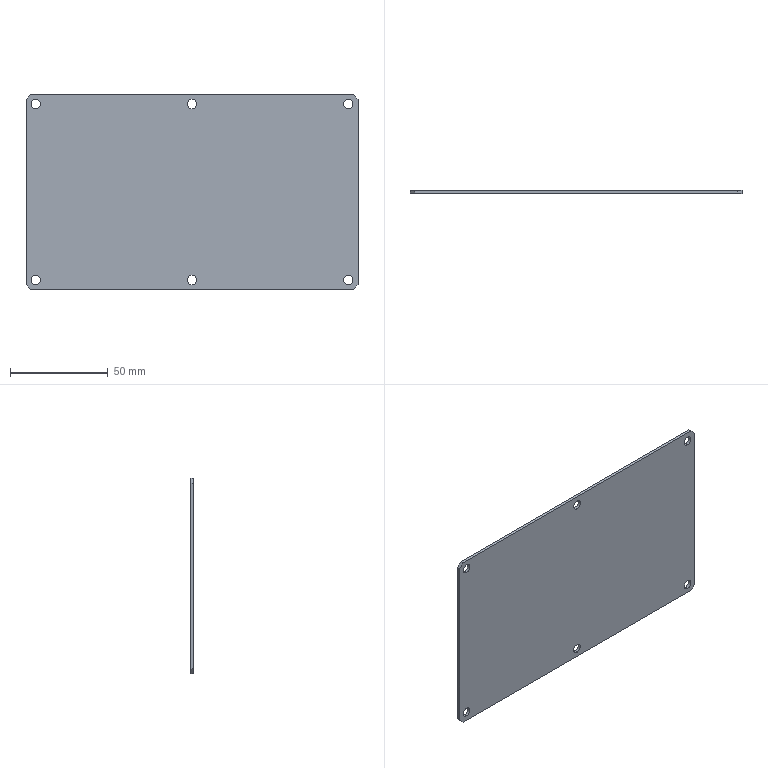Part | SolidWorks | features BreakCorner 1, FlatPattern 1, HoleWzd 1, SMBaseFlange 1, SheetMetal 1 | 1 solid | 22 faces | box 170 x 1.5 x 100 mm | volume 25318 mm3 | cylinder 12 | plane 10 | commonest cylinder face diameters 4.8 x12
STEP:
#1=CARTESIAN_POINT('',(80.,0.,-42.6));
#2=VERTEX_POINT('',#1);
#3=CARTESIAN_POINT('',(80.,0.,-47.4));
#4=VERTEX_POINT('',#3);
#5=CARTESIAN_POINT('',(80.,0.,-45.));
#6=DIRECTION('',(0.,-1.,0.));
#7=DIRECTION('',(0.,0.,-1.));
#8=AXIS2_PLACEMENT_3D('',#5,#6,#7);
#9=CIRCLE('',#8,2.4);
#10=EDGE_CURVE('',#2,#4,#9,.T.);
#11=ORIENTED_EDGE('',*,*,#10,.F.);
#12=CARTESIAN_POINT('',(80.,-1.5,-42.6));
#13=VERTEX_POINT('',#12);
#14=CARTESIAN_POINT('',(80.,-1.5,-42.6));
#15=DIRECTION('',(0.,-1.,0.));
#16=VECTOR('',#15,1000.);
#17=LINE('',#14,#16);
#18=EDGE_CURVE('',#2,#13,#17,.T.);
#19=ORIENTED_EDGE('',*,*,#18,.T.);
#20=CARTESIAN_POINT('',(80.,-1.5,-47.4));
#21=VERTEX_POINT('',#20);
#22=CARTESIAN_POINT('',(80.,-1.5,-45.));
#23=DIRECTION('',(0.,-1.,0.));
#24=DIRECTION('',(0.,0.,-1.));
#25=AXIS2_PLACEMENT_3D('',#22,#23,#24);
#26=CIRCLE('',#25,2.4);
#27=EDGE_CURVE('',#13,#21,#26,.T.);
#28=ORIENTED_EDGE('',*,*,#27,.T.);
#29=CARTESIAN_POINT('',(80.,-1.5,-47.4));
#30=DIRECTION('',(0.,-1.,0.));
#31=VECTOR('',#30,1000.);
#32=LINE('',#29,#31);
#33=EDGE_CURVE('',#4,#21,#32,.T.);
#34=ORIENTED_EDGE('',*,*,#33,.F.);
#35=EDGE_LOOP('',(#11,#19,#28,#34));
#36=FACE_OUTER_BOUND('',#35,.T.);
#37=CARTESIAN_POINT('',(80.,-1.5,-45.));
#38=DIRECTION('',(0.,-1.,0.));
#39=DIRECTION('',(0.,0.,-1.));
#40=AXIS2_PLACEMENT_3D('',#37,#38,#39);
#41=CYLINDRICAL_SURFACE('',#40,2.4);
#42=ADVANCED_FACE('',(#36),#41,.F.);
#43=CARTESIAN_POINT('',(0.,0.,-42.6));
#44=VERTEX_POINT('',#43);
#45=CARTESIAN_POINT('',(0.,0.,-47.4));
#46=VERTEX_POINT('',#45);
#47=CARTESIAN_POINT('',(0.,0.,-45.));
#48=DIRECTION('',(0.,-1.,0.));
#49=DIRECTION('',(0.,0.,-1.));
#50=AXIS2_PLACEMENT_3D('',#47,#48,#49);
#51=CIRCLE('',#50,2.4);
#52=EDGE_CURVE('',#44,#46,#51,.T.);
#53=ORIENTED_EDGE('',*,*,#52,.F.);
#54=CARTESIAN_POINT('',(0.,-1.5,-42.6));
#55=VERTEX_POINT('',#54);
#56=CARTESIAN_POINT('',(0.,-1.5,-42.6));
#57=DIRECTION('',(0.,-1.,0.));
#58=VECTOR('',#57,1000.);
#59=LINE('',#56,#58);
#60=EDGE_CURVE('',#44,#55,#59,.T.);
#61=ORIENTED_EDGE('',*,*,#60,.T.);
#62=CARTESIAN_POINT('',(0.,-1.5,-47.4));
#63=VERTEX_POINT('',#62);
#64=CARTESIAN_POINT('',(0.,-1.5,-45.));
#65=DIRECTION('',(0.,-1.,0.));
#66=DIRECTION('',(0.,0.,-1.));
#67=AXIS2_PLACEMENT_3D('',#64,#65,#66);
#68=CIRCLE('',#67,2.4);
#69=EDGE_CURVE('',#55,#63,#68,.T.);
#70=ORIENTED_EDGE('',*,*,#69,.T.);
#71=CARTESIAN_POINT('',(0.,-1.5,-47.4));
#72=DIRECTION('',(0.,-1.,0.));
#73=VECTOR('',#72,1000.);
#74=LINE('',#71,#73);
#75=EDGE_CURVE('',#46,#63,#74,.T.);
#76=ORIENTED_EDGE('',*,*,#75,.F.);
#77=EDGE_LOOP('',(#53,#61,#70,#76));
#78=FACE_OUTER_BOUND('',#77,.T.);
#79=CARTESIAN_POINT('',(0.,-1.5,-45.));
#80=DIRECTION('',(0.,-1.,0.));
#81=DIRECTION('',(0.,0.,-1.));
#82=AXIS2_PLACEMENT_3D('',#79,#80,#81);
#83=CYLINDRICAL_SURFACE('',#82,2.4);
#84=ADVANCED_FACE('',(#78),#83,.F.);
#85=CARTESIAN_POINT('',(-80.,0.,-42.6));
#86=VERTEX_POINT('',#85);
#87=CARTESIAN_POINT('',(-80.,0.,-47.4));
#88=VERTEX_POINT('',#87);
#89=CARTESIAN_POINT('',(-80.,0.,-45.));
#90=DIRECTION('',(0.,-1.,0.));
#91=DIRECTION('',(0.,0.,-1.));
#92=AXIS2_PLACEMENT_3D('',#89,#90,#91);
#93=CIRCLE('',#92,2.4);
#94=EDGE_CURVE('',#86,#88,#93,.T.);
#95=ORIENTED_EDGE('',*,*,#94,.F.);
#96=CARTESIAN_POINT('',(-80.,-1.5,-42.6));
#97=VERTEX_POINT('',#96);
#98=CARTESIAN_POINT('',(-80.,-1.5,-42.6));
#99=DIRECTION('',(0.,-1.,0.));
#100=VECTOR('',#99,1000.);
#101=LINE('',#98,#100);
#102=EDGE_CURVE('',#86,#97,#101,.T.);
#103=ORIENTED_EDGE('',*,*,#102,.T.);
#104=CARTESIAN_POINT('',(-80.,-1.5,-47.4));
#105=VERTEX_POINT('',#104);
#106=CARTESIAN_POINT('',(-80.,-1.5,-45.));
#107=DIRECTION('',(0.,-1.,0.));
#108=DIRECTION('',(0.,0.,-1.));
#109=AXIS2_PLACEMENT_3D('',#106,#107,#108);
#110=CIRCLE('',#109,2.4);
#111=EDGE_CURVE('',#97,#105,#110,.T.);
#112=ORIENTED_EDGE('',*,*,#111,.T.);
#113=CARTESIAN_POINT('',(-80.,-1.5,-47.4));
#114=DIRECTION('',(0.,-1.,0.));
#115=VECTOR('',#114,1000.);
#116=LINE('',#113,#115);
#117=EDGE_CURVE('',#88,#105,#116,.T.);
#118=ORIENTED_EDGE('',*,*,#117,.F.);
#119=EDGE_LOOP('',(#95,#103,#112,#118));
#120=FACE_OUTER_BOUND('',#119,.T.);
#121=CARTESIAN_POINT('',(-80.,-1.5,-45.));
#122=DIRECTION('',(0.,-1.,0.));
#123=DIRECTION('',(0.,0.,-1.));
#124=AXIS2_PLACEMENT_3D('',#121,#122,#123);
#125=CYLINDRICAL_SURFACE('',#124,2.4);
#126=ADVANCED_FACE('',(#120),#125,.F.);
#127=CARTESIAN_POINT('',(-80.,0.,47.4));
#128=VERTEX_POINT('',#127);
#129=CARTESIAN_POINT('',(-80.,0.,42.6));
#130=VERTEX_POINT('',#129);
#131=CARTESIAN_POINT('',(-80.,0.,45.));
#132=DIRECTION('',(0.,-1.,0.));
#133=DIRECTION('',(0.,0.,-1.));
#134=AXIS2_PLACEMENT_3D('',#131,#132,#133);
#135=CIRCLE('',#134,2.4);
#136=EDGE_CURVE('',#128,#130,#135,.T.);
#137=ORIENTED_EDGE('',*,*,#136,.F.);
#138=CARTESIAN_POINT('',(-80.,-1.5,47.4));
#139=VERTEX_POINT('',#138);
#140=CARTESIAN_POINT('',(-80.,-1.5,47.4));
#141=DIRECTION('',(0.,-1.,0.));
#142=VECTOR('',#141,1000.);
#143=LINE('',#140,#142);
#144=EDGE_CURVE('',#128,#139,#143,.T.);
#145=ORIENTED_EDGE('',*,*,#144,.T.);
#146=CARTESIAN_POINT('',(-80.,-1.5,42.6));
#147=VERTEX_POINT('',#146);
#148=CARTESIAN_POINT('',(-80.,-1.5,45.));
#149=DIRECTION('',(0.,-1.,0.));
#150=DIRECTION('',(0.,0.,-1.));
#151=AXIS2_PLACEMENT_3D('',#148,#149,#150);
#152=CIRCLE('',#151,2.4);
#153=EDGE_CURVE('',#139,#147,#152,.T.);
#154=ORIENTED_EDGE('',*,*,#153,.T.);
#155=CARTESIAN_POINT('',(-80.,-1.5,42.6));
#156=DIRECTION('',(0.,-1.,0.));
#157=VECTOR('',#156,1000.);
#158=LINE('',#155,#157);
#159=EDGE_CURVE('',#130,#147,#158,.T.);
#160=ORIENTED_EDGE('',*,*,#159,.F.);
#161=EDGE_LOOP('',(#137,#145,#154,#160));
#162=FACE_OUTER_BOUND('',#161,.T.);
#163=CARTESIAN_POINT('',(-80.,-1.5,45.));
#164=DIRECTION('',(0.,-1.,0.));
#165=DIRECTION('',(0.,0.,-1.));
#166=AXIS2_PLACEMENT_3D('',#163,#164,#165);
#167=CYLINDRICAL_SURFACE('',#166,2.4);
#168=ADVANCED_FACE('',(#162),#167,.F.);
#169=CARTESIAN_POINT('',(0.,0.,47.4));
#170=VERTEX_POINT('',#169);
#171=CARTESIAN_POINT('',(0.,0.,42.6));
#172=VERTEX_POINT('',#171);
#173=CARTESIAN_POINT('',(0.,0.,45.));
#174=DIRECTION('',(0.,-1.,0.));
#175=DIRECTION('',(0.,0.,-1.));
#176=AXIS2_PLACEMENT_3D('',#173,#174,#175);
#177=CIRCLE('',#176,2.4);
#178=EDGE_CURVE('',#170,#172,#177,.T.);
#179=ORIENTED_EDGE('',*,*,#178,.F.);
#180=CARTESIAN_POINT('',(0.,-1.5,47.4));
#181=VERTEX_POINT('',#180);
#182=CARTESIAN_POINT('',(0.,-1.5,47.4));
#183=DIRECTION('',(0.,-1.,0.));
#184=VECTOR('',#183,1000.);
#185=LINE('',#182,#184);
#186=EDGE_CURVE('',#170,#181,#185,.T.);
#187=ORIENTED_EDGE('',*,*,#186,.T.);
#188=CARTESIAN_POINT('',(0.,-1.5,42.6));
#189=VERTEX_POINT('',#188);
#190=CARTESIAN_POINT('',(0.,-1.5,45.));
#191=DIRECTION('',(0.,-1.,0.));
#192=DIRECTION('',(0.,0.,-1.));
#193=AXIS2_PLACEMENT_3D('',#190,#191,#192);
#194=CIRCLE('',#193,2.4);
#195=EDGE_CURVE('',#181,#189,#194,.T.);
#196=ORIENTED_EDGE('',*,*,#195,.T.);
#197=CARTESIAN_POINT('',(0.,-1.5,42.6));
#198=DIRECTION('',(0.,-1.,0.));
#199=VECTOR('',#198,1000.);
#200=LINE('',#197,#199);
#201=EDGE_CURVE('',#172,#189,#200,.T.);
#202=ORIENTED_EDGE('',*,*,#201,.F.);
#203=EDGE_LOOP('',(#179,#187,#196,#202));
#204=FACE_OUTER_BOUND('',#203,.T.);
#205=CARTESIAN_POINT('',(0.,-1.5,45.));
#206=DIRECTION('',(0.,-1.,0.));
#207=DIRECTION('',(0.,0.,-1.));
#208=AXIS2_PLACEMENT_3D('',#205,#206,#207);
#209=CYLINDRICAL_SURFACE('',#208,2.4);
#210=ADVANCED_FACE('',(#204),#209,.F.);
#211=CARTESIAN_POINT('',(80.,0.,47.4));
#212=VERTEX_POINT('',#211);
#213=CARTESIAN_POINT('',(80.,0.,42.6));
#214=VERTEX_POINT('',#213);
#215=CARTESIAN_POINT('',(80.,0.,45.));
#216=DIRECTION('',(0.,-1.,0.));
#217=DIRECTION('',(0.,0.,-1.));
#218=AXIS2_PLACEMENT_3D('',#215,#216,#217);
#219=CIRCLE('',#218,2.4);
#220=EDGE_CURVE('',#212,#214,#219,.T.);
#221=ORIENTED_EDGE('',*,*,#220,.F.);
#222=CARTESIAN_POINT('',(80.,-1.5,47.4));
#223=VERTEX_POINT('',#222);
#224=CARTESIAN_POINT('',(80.,-1.5,47.4));
#225=DIRECTION('',(0.,-1.,0.));
#226=VECTOR('',#225,1000.);
#227=LINE('',#224,#226);
#228=EDGE_CURVE('',#212,#223,#227,.T.);
#229=ORIENTED_EDGE('',*,*,#228,.T.);
#230=CARTESIAN_POINT('',(80.,-1.5,42.6));
#231=VERTEX_POINT('',#230);
#232=CARTESIAN_POINT('',(80.,-1.5,45.));
#233=DIRECTION('',(0.,-1.,0.));
#234=DIRECTION('',(0.,0.,-1.));
#235=AXIS2_PLACEMENT_3D('',#232,#233,#234);
#236=CIRCLE('',#235,2.4);
#237=EDGE_CURVE('',#223,#231,#236,.T.);
#238=ORIENTED_EDGE('',*,*,#237,.T.);
#239=CARTESIAN_POINT('',(80.,-1.5,42.6));
#240=DIRECTION('',(0.,-1.,0.));
#241=VECTOR('',#240,1000.);
#242=LINE('',#239,#241);
#243=EDGE_CURVE('',#214,#231,#242,.T.);
#244=ORIENTED_EDGE('',*,*,#243,.F.);
#245=EDGE_LOOP('',(#221,#229,#238,#244));
#246=FACE_OUTER_BOUND('',#245,.T.);
#247=CARTESIAN_POINT('',(80.,-1.5,45.));
#248=DIRECTION('',(0.,-1.,0.));
#249=DIRECTION('',(0.,0.,-1.));
#250=AXIS2_PLACEMENT_3D('',#247,#248,#249);
#251=CYLINDRICAL_SURFACE('',#250,2.4);
#252=ADVANCED_FACE('',(#246),#251,.F.);
#253=CARTESIAN_POINT('',(85.,-1.5,47.5));
#254=VERTEX_POINT('',#253);
#255=CARTESIAN_POINT('',(85.,-1.5,-47.5));
#256=VERTEX_POINT('',#255);
#257=CARTESIAN_POINT('',(85.,-1.5,50.));
#258=DIRECTION('',(0.,0.,-1.));
#259=VECTOR('',#258,1000.);
#260=LINE('',#257,#259);
#261=EDGE_CURVE('',#254,#256,#260,.T.);
#262=ORIENTED_EDGE('',*,*,#261,.T.);
#263=CARTESIAN_POINT('',(85.,0.,-47.5));
#264=VERTEX_POINT('',#263);
#265=CARTESIAN_POINT('',(85.,-1.5,-47.5));
#266=DIRECTION('',(0.,1.,0.));
#267=VECTOR('',#266,1000.);
#268=LINE('',#265,#267);
#269=EDGE_CURVE('',#256,#264,#268,.T.);
#270=ORIENTED_EDGE('',*,*,#269,.T.);
#271=CARTESIAN_POINT('',(85.,0.,47.5));
#272=VERTEX_POINT('',#271);
#273=CARTESIAN_POINT('',(85.,0.,50.));
#274=DIRECTION('',(0.,0.,-1.));
#275=VECTOR('',#274,1000.);
#276=LINE('',#273,#275);
#277=EDGE_CURVE('',#272,#264,#276,.T.);
#278=ORIENTED_EDGE('',*,*,#277,.F.);
#279=CARTESIAN_POINT('',(85.,-1.5,47.5));
#280=DIRECTION('',(0.,-1.,0.));
#281=VECTOR('',#280,1000.);
#282=LINE('',#279,#281);
#283=EDGE_CURVE('',#272,#254,#282,.T.);
#284=ORIENTED_EDGE('',*,*,#283,.T.);
#285=EDGE_LOOP('',(#262,#270,#278,#284));
#286=FACE_OUTER_BOUND('',#285,.T.);
#287=CARTESIAN_POINT('',(85.,-1.5,50.));
#288=DIRECTION('',(1.,0.,0.));
#289=DIRECTION('',(0.,0.,-1.));
#290=AXIS2_PLACEMENT_3D('',#287,#288,#289);
#291=PLANE('',#290);
#292=ADVANCED_FACE('',(#286),#291,.T.);
#293=CARTESIAN_POINT('',(-82.5,0.,50.));
#294=VERTEX_POINT('',#293);
#295=CARTESIAN_POINT('',(82.5,0.,50.));
#296=VERTEX_POINT('',#295);
#297=CARTESIAN_POINT('',(-85.,0.,50.));
#298=DIRECTION('',(1.,0.,0.));
#299=VECTOR('',#298,1000.);
#300=LINE('',#297,#299);
#301=EDGE_CURVE('',#294,#296,#300,.T.);
#302=ORIENTED_EDGE('',*,*,#301,.F.);
#303=CARTESIAN_POINT('',(-82.5,-1.5,50.));
#304=VERTEX_POINT('',#303);
#305=CARTESIAN_POINT('',(-82.5,-1.5,50.));
#306=DIRECTION('',(0.,-1.,0.));
#307=VECTOR('',#306,1000.);
#308=LINE('',#305,#307);
#309=EDGE_CURVE('',#294,#304,#308,.T.);
#310=ORIENTED_EDGE('',*,*,#309,.T.);
#311=CARTESIAN_POINT('',(82.5,-1.5,50.));
#312=VERTEX_POINT('',#311);
#313=CARTESIAN_POINT('',(-85.,-1.5,50.));
#314=DIRECTION('',(1.,0.,0.));
#315=VECTOR('',#314,1000.);
#316=LINE('',#313,#315);
#317=EDGE_CURVE('',#304,#312,#316,.T.);
#318=ORIENTED_EDGE('',*,*,#317,.T.);
#319=CARTESIAN_POINT('',(82.5,-1.5,50.));
#320=DIRECTION('',(0.,1.,0.));
#321=VECTOR('',#320,1000.);
#322=LINE('',#319,#321);
#323=EDGE_CURVE('',#312,#296,#322,.T.);
#324=ORIENTED_EDGE('',*,*,#323,.T.);
#325=EDGE_LOOP('',(#302,#310,#318,#324));
#326=FACE_OUTER_BOUND('',#325,.T.);
#327=CARTESIAN_POINT('',(-85.,-1.5,50.));
#328=DIRECTION('',(0.,0.,1.));
#329=DIRECTION('',(1.,0.,0.));
#330=AXIS2_PLACEMENT_3D('',#327,#328,#329);
#331=PLANE('',#330);
#332=ADVANCED_FACE('',(#326),#331,.T.);
#333=CARTESIAN_POINT('',(-85.,0.,-47.5));
#334=VERTEX_POINT('',#333);
#335=CARTESIAN_POINT('',(-85.,0.,47.5));
#336=VERTEX_POINT('',#335);
#337=CARTESIAN_POINT('',(-85.,0.,50.));
#338=DIRECTION('',(0.,0.,1.));
#339=VECTOR('',#338,1000.);
#340=LINE('',#337,#339);
#341=EDGE_CURVE('',#334,#336,#340,.T.);
#342=ORIENTED_EDGE('',*,*,#341,.F.);
#343=CARTESIAN_POINT('',(-85.,-1.5,-47.5));
#344=VERTEX_POINT('',#343);
#345=CARTESIAN_POINT('',(-85.,-1.5,-47.5));
#346=DIRECTION('',(0.,-1.,0.));
#347=VECTOR('',#346,1000.);
#348=LINE('',#345,#347);
#349=EDGE_CURVE('',#334,#344,#348,.T.);
#350=ORIENTED_EDGE('',*,*,#349,.T.);
#351=CARTESIAN_POINT('',(-85.,-1.5,47.5));
#352=VERTEX_POINT('',#351);
#353=CARTESIAN_POINT('',(-85.,-1.5,50.));
#354=DIRECTION('',(0.,0.,1.));
#355=VECTOR('',#354,1000.);
#356=LINE('',#353,#355);
#357=EDGE_CURVE('',#344,#352,#356,.T.);
#358=ORIENTED_EDGE('',*,*,#357,.T.);
#359=CARTESIAN_POINT('',(-85.,-1.5,47.5));
#360=DIRECTION('',(0.,1.,0.));
#361=VECTOR('',#360,1000.);
#362=LINE('',#359,#361);
#363=EDGE_CURVE('',#352,#336,#362,.T.);
#364=ORIENTED_EDGE('',*,*,#363,.T.);
#365=EDGE_LOOP('',(#342,#350,#358,#364));
#366=FACE_OUTER_BOUND('',#365,.T.);
#367=CARTESIAN_POINT('',(-85.,-1.5,50.));
#368=DIRECTION('',(-1.,0.,0.));
#369=DIRECTION('',(0.,0.,1.));
#370=AXIS2_PLACEMENT_3D('',#367,#368,#369);
#371=PLANE('',#370);
#372=ADVANCED_FACE('',(#366),#371,.T.);
#373=CARTESIAN_POINT('',(82.5,0.,-50.));
#374=VERTEX_POINT('',#373);
#375=CARTESIAN_POINT('',(-82.5,0.,-50.));
#376=VERTEX_POINT('',#375);
#377=CARTESIAN_POINT('',(-85.,0.,-50.));
#378=DIRECTION('',(-1.,0.,0.));
#379=VECTOR('',#378,1000.);
#380=LINE('',#377,#379);
#381=EDGE_CURVE('',#374,#376,#380,.T.);
#382=ORIENTED_EDGE('',*,*,#381,.F.);
#383=CARTESIAN_POINT('',(82.5,-1.5,-50.));
#384=VERTEX_POINT('',#383);
#385=CARTESIAN_POINT('',(82.5,-1.5,-50.));
#386=DIRECTION('',(0.,-1.,0.));
#387=VECTOR('',#386,1000.);
#388=LINE('',#385,#387);
#389=EDGE_CURVE('',#374,#384,#388,.T.);
#390=ORIENTED_EDGE('',*,*,#389,.T.);
#391=CARTESIAN_POINT('',(-82.5,-1.5,-50.));
#392=VERTEX_POINT('',#391);
#393=CARTESIAN_POINT('',(-85.,-1.5,-50.));
#394=DIRECTION('',(-1.,0.,0.));
#395=VECTOR('',#394,1000.);
#396=LINE('',#393,#395);
#397=EDGE_CURVE('',#384,#392,#396,.T.);
#398=ORIENTED_EDGE('',*,*,#397,.T.);
#399=CARTESIAN_POINT('',(-82.5,-1.5,-50.));
#400=DIRECTION('',(0.,1.,0.));
#401=VECTOR('',#400,1000.);
#402=LINE('',#399,#401);
#403=EDGE_CURVE('',#392,#376,#402,.T.);
#404=ORIENTED_EDGE('',*,*,#403,.T.);
#405=EDGE_LOOP('',(#382,#390,#398,#404));
#406=FACE_OUTER_BOUND('',#405,.T.);
#407=CARTESIAN_POINT('',(-85.,-1.5,-50.));
#408=DIRECTION('',(0.,0.,-1.));
#409=DIRECTION('',(-1.,0.,0.));
#410=AXIS2_PLACEMENT_3D('',#407,#408,#409);
#411=PLANE('',#410);
#412=ADVANCED_FACE('',(#406),#411,.T.);
#413=CARTESIAN_POINT('',(80.,-1.5,-45.));
#414=DIRECTION('',(0.,-1.,0.));
#415=DIRECTION('',(0.,0.,-1.));
#416=AXIS2_PLACEMENT_3D('',#413,#414,#415);
#417=CIRCLE('',#416,2.4);
#418=EDGE_CURVE('',#21,#13,#417,.T.);
#419=ORIENTED_EDGE('',*,*,#418,.F.);
#420=ORIENTED_EDGE('',*,*,#27,.F.);
#421=EDGE_LOOP('',(#419,#420));
#422=FACE_BOUND('',#421,.T.);
#423=CARTESIAN_POINT('',(0.,-1.5,-45.));
#424=DIRECTION('',(0.,-1.,0.));
#425=DIRECTION('',(0.,0.,-1.));
#426=AXIS2_PLACEMENT_3D('',#423,#424,#425);
#427=CIRCLE('',#426,2.4);
#428=EDGE_CURVE('',#63,#55,#427,.T.);
#429=ORIENTED_EDGE('',*,*,#428,.F.);
#430=ORIENTED_EDGE('',*,*,#69,.F.);
#431=EDGE_LOOP('',(#429,#430));
#432=FACE_BOUND('',#431,.T.);
#433=CARTESIAN_POINT('',(-80.,-1.5,-45.));
#434=DIRECTION('',(0.,-1.,0.));
#435=DIRECTION('',(0.,0.,-1.));
#436=AXIS2_PLACEMENT_3D('',#433,#434,#435);
#437=CIRCLE('',#436,2.4);
#438=EDGE_CURVE('',#105,#97,#437,.T.);
#439=ORIENTED_EDGE('',*,*,#438,.F.);
#440=ORIENTED_EDGE('',*,*,#111,.F.);
#441=EDGE_LOOP('',(#439,#440));
#442=FACE_BOUND('',#441,.T.);
#443=CARTESIAN_POINT('',(-80.,-1.5,45.));
#444=DIRECTION('',(0.,-1.,0.));
#445=DIRECTION('',(0.,0.,-1.));
#446=AXIS2_PLACEMENT_3D('',#443,#444,#445);
#447=CIRCLE('',#446,2.4);
#448=EDGE_CURVE('',#147,#139,#447,.T.);
#449=ORIENTED_EDGE('',*,*,#448,.F.);
#450=ORIENTED_EDGE('',*,*,#153,.F.);
#451=EDGE_LOOP('',(#449,#450));
#452=FACE_BOUND('',#451,.T.);
#453=CARTESIAN_POINT('',(0.,-1.5,45.));
#454=DIRECTION('',(0.,-1.,0.));
#455=DIRECTION('',(0.,0.,-1.));
#456=AXIS2_PLACEMENT_3D('',#453,#454,#455);
#457=CIRCLE('',#456,2.4);
#458=EDGE_CURVE('',#189,#181,#457,.T.);
#459=ORIENTED_EDGE('',*,*,#458,.F.);
#460=ORIENTED_EDGE('',*,*,#195,.F.);
#461=EDGE_LOOP('',(#459,#460));
#462=FACE_BOUND('',#461,.T.);
#463=CARTESIAN_POINT('',(80.,-1.5,45.));
#464=DIRECTION('',(0.,-1.,0.));
#465=DIRECTION('',(0.,0.,-1.));
#466=AXIS2_PLACEMENT_3D('',#463,#464,#465);
#467=CIRCLE('',#466,2.4);
#468=EDGE_CURVE('',#231,#223,#467,.T.);
#469=ORIENTED_EDGE('',*,*,#468,.F.);
#470=ORIENTED_EDGE('',*,*,#237,.F.);
#471=EDGE_LOOP('',(#469,#470));
#472=FACE_BOUND('',#471,.T.);
#473=ORIENTED_EDGE('',*,*,#397,.F.);
#474=CARTESIAN_POINT('',(66.25,-1.5,-66.25));
#475=DIRECTION('',(0.7071,0.,0.7071));
#476=VECTOR('',#475,1000.);
#477=LINE('',#474,#476);
#478=EDGE_CURVE('',#384,#256,#477,.T.);
#479=ORIENTED_EDGE('',*,*,#478,.T.);
#480=ORIENTED_EDGE('',*,*,#261,.F.);
#481=CARTESIAN_POINT('',(66.25,-1.5,66.25));
#482=DIRECTION('',(-0.7071,0.,0.7071));
#483=VECTOR('',#482,1000.);
#484=LINE('',#481,#483);
#485=EDGE_CURVE('',#254,#312,#484,.T.);
#486=ORIENTED_EDGE('',*,*,#485,.T.);
#487=ORIENTED_EDGE('',*,*,#317,.F.);
#488=CARTESIAN_POINT('',(-66.25,-1.5,66.25));
#489=DIRECTION('',(-0.7071,0.,-0.7071));
#490=VECTOR('',#489,1000.);
#491=LINE('',#488,#490);
#492=EDGE_CURVE('',#304,#352,#491,.T.);
#493=ORIENTED_EDGE('',*,*,#492,.T.);
#494=ORIENTED_EDGE('',*,*,#357,.F.);
#495=CARTESIAN_POINT('',(-66.25,-1.5,-66.25));
#496=DIRECTION('',(0.7071,0.,-0.7071));
#497=VECTOR('',#496,1000.);
#498=LINE('',#495,#497);
#499=EDGE_CURVE('',#344,#392,#498,.T.);
#500=ORIENTED_EDGE('',*,*,#499,.T.);
#501=EDGE_LOOP('',(#473,#479,#480,#486,#487,#493,#494,#500));
#502=FACE_OUTER_BOUND('',#501,.T.);
#503=CARTESIAN_POINT('',(0.,-1.5,0.));
#504=DIRECTION('',(0.,-1.,0.));
#505=DIRECTION('',(0.,0.,-1.));
#506=AXIS2_PLACEMENT_3D('',#503,#504,#505);
#507=PLANE('',#506);
#508=ADVANCED_FACE('',(#422,#432,#442,#452,#462,#472,#502),#507,.T.);
#509=CARTESIAN_POINT('',(80.,0.,-45.));
#510=DIRECTION('',(0.,-1.,0.));
#511=DIRECTION('',(0.,0.,-1.));
#512=AXIS2_PLACEMENT_3D('',#509,#510,#511);
#513=CIRCLE('',#512,2.4);
#514=EDGE_CURVE('',#4,#2,#513,.T.);
#515=ORIENTED_EDGE('',*,*,#514,.T.);
#516=ORIENTED_EDGE('',*,*,#10,.T.);
#517=EDGE_LOOP('',(#515,#516));
#518=FACE_BOUND('',#517,.T.);
#519=CARTESIAN_POINT('',(0.,0.,-45.));
#520=DIRECTION('',(0.,-1.,0.));
#521=DIRECTION('',(0.,0.,-1.));
#522=AXIS2_PLACEMENT_3D('',#519,#520,#521);
#523=CIRCLE('',#522,2.4);
#524=EDGE_CURVE('',#46,#44,#523,.T.);
#525=ORIENTED_EDGE('',*,*,#524,.T.);
#526=ORIENTED_EDGE('',*,*,#52,.T.);
#527=EDGE_LOOP('',(#525,#526));
#528=FACE_BOUND('',#527,.T.);
#529=CARTESIAN_POINT('',(-80.,0.,-45.));
#530=DIRECTION('',(0.,-1.,0.));
#531=DIRECTION('',(0.,0.,-1.));
#532=AXIS2_PLACEMENT_3D('',#529,#530,#531);
#533=CIRCLE('',#532,2.4);
#534=EDGE_CURVE('',#88,#86,#533,.T.);
#535=ORIENTED_EDGE('',*,*,#534,.T.);
#536=ORIENTED_EDGE('',*,*,#94,.T.);
#537=EDGE_LOOP('',(#535,#536));
#538=FACE_BOUND('',#537,.T.);
#539=CARTESIAN_POINT('',(-80.,0.,45.));
#540=DIRECTION('',(0.,-1.,0.));
#541=DIRECTION('',(0.,0.,-1.));
#542=AXIS2_PLACEMENT_3D('',#539,#540,#541);
#543=CIRCLE('',#542,2.4);
#544=EDGE_CURVE('',#130,#128,#543,.T.);
#545=ORIENTED_EDGE('',*,*,#544,.T.);
#546=ORIENTED_EDGE('',*,*,#136,.T.);
#547=EDGE_LOOP('',(#545,#546));
#548=FACE_BOUND('',#547,.T.);
#549=CARTESIAN_POINT('',(0.,0.,45.));
#550=DIRECTION('',(0.,-1.,0.));
#551=DIRECTION('',(0.,0.,-1.));
#552=AXIS2_PLACEMENT_3D('',#549,#550,#551);
#553=CIRCLE('',#552,2.4);
#554=EDGE_CURVE('',#172,#170,#553,.T.);
#555=ORIENTED_EDGE('',*,*,#554,.T.);
#556=ORIENTED_EDGE('',*,*,#178,.T.);
#557=EDGE_LOOP('',(#555,#556));
#558=FACE_BOUND('',#557,.T.);
#559=CARTESIAN_POINT('',(80.,0.,45.));
#560=DIRECTION('',(0.,-1.,0.));
#561=DIRECTION('',(0.,0.,-1.));
#562=AXIS2_PLACEMENT_3D('',#559,#560,#561);
#563=CIRCLE('',#562,2.4);
#564=EDGE_CURVE('',#214,#212,#563,.T.);
#565=ORIENTED_EDGE('',*,*,#564,.T.);
#566=ORIENTED_EDGE('',*,*,#220,.T.);
#567=EDGE_LOOP('',(#565,#566));
#568=FACE_BOUND('',#567,.T.);
#569=ORIENTED_EDGE('',*,*,#277,.T.);
#570=CARTESIAN_POINT('',(85.,0.,-47.5));
#571=DIRECTION('',(-0.7071,0.,-0.7071));
#572=VECTOR('',#571,1000.);
#573=LINE('',#570,#572);
#574=EDGE_CURVE('',#264,#374,#573,.T.);
#575=ORIENTED_EDGE('',*,*,#574,.T.);
#576=ORIENTED_EDGE('',*,*,#381,.T.);
#577=CARTESIAN_POINT('',(-82.5,0.,-50.));
#578=DIRECTION('',(-0.7071,0.,0.7071));
#579=VECTOR('',#578,1000.);
#580=LINE('',#577,#579);
#581=EDGE_CURVE('',#376,#334,#580,.T.);
#582=ORIENTED_EDGE('',*,*,#581,.T.);
#583=ORIENTED_EDGE('',*,*,#341,.T.);
#584=CARTESIAN_POINT('',(-85.,0.,47.5));
#585=DIRECTION('',(0.7071,0.,0.7071));
#586=VECTOR('',#585,1000.);
#587=LINE('',#584,#586);
#588=EDGE_CURVE('',#336,#294,#587,.T.);
#589=ORIENTED_EDGE('',*,*,#588,.T.);
#590=ORIENTED_EDGE('',*,*,#301,.T.);
#591=CARTESIAN_POINT('',(82.5,0.,50.));
#592=DIRECTION('',(0.7071,0.,-0.7071));
#593=VECTOR('',#592,1000.);
#594=LINE('',#591,#593);
#595=EDGE_CURVE('',#296,#272,#594,.T.);
#596=ORIENTED_EDGE('',*,*,#595,.T.);
#597=EDGE_LOOP('',(#569,#575,#576,#582,#583,#589,#590,#596));
#598=FACE_OUTER_BOUND('',#597,.T.);
#599=CARTESIAN_POINT('',(0.,0.,0.));
#600=DIRECTION('',(0.,-1.,0.));
#601=DIRECTION('',(0.,0.,-1.));
#602=AXIS2_PLACEMENT_3D('',#599,#600,#601);
#603=PLANE('',#602);
#604=ADVANCED_FACE('',(#518,#528,#538,#548,#558,#568,#598),#603,.F.);
#605=ORIENTED_EDGE('',*,*,#228,.F.);
#606=ORIENTED_EDGE('',*,*,#564,.F.);
#607=ORIENTED_EDGE('',*,*,#243,.T.);
#608=ORIENTED_EDGE('',*,*,#468,.T.);
#609=EDGE_LOOP('',(#605,#606,#607,#608));
#610=FACE_OUTER_BOUND('',#609,.T.);
#611=CARTESIAN_POINT('',(80.,-1.5,45.));
#612=DIRECTION('',(0.,-1.,0.));
#613=DIRECTION('',(0.,0.,-1.));
#614=AXIS2_PLACEMENT_3D('',#611,#612,#613);
#615=CYLINDRICAL_SURFACE('',#614,2.4);
#616=ADVANCED_FACE('',(#610),#615,.F.);
#617=ORIENTED_EDGE('',*,*,#186,.F.);
#618=ORIENTED_EDGE('',*,*,#554,.F.);
#619=ORIENTED_EDGE('',*,*,#201,.T.);
#620=ORIENTED_EDGE('',*,*,#458,.T.);
#621=EDGE_LOOP('',(#617,#618,#619,#620));
#622=FACE_OUTER_BOUND('',#621,.T.);
#623=CARTESIAN_POINT('',(0.,-1.5,45.));
#624=DIRECTION('',(0.,-1.,0.));
#625=DIRECTION('',(0.,0.,-1.));
#626=AXIS2_PLACEMENT_3D('',#623,#624,#625);
#627=CYLINDRICAL_SURFACE('',#626,2.4);
#628=ADVANCED_FACE('',(#622),#627,.F.);
#629=ORIENTED_EDGE('',*,*,#144,.F.);
#630=ORIENTED_EDGE('',*,*,#544,.F.);
#631=ORIENTED_EDGE('',*,*,#159,.T.);
#632=ORIENTED_EDGE('',*,*,#448,.T.);
#633=EDGE_LOOP('',(#629,#630,#631,#632));
#634=FACE_OUTER_BOUND('',#633,.T.);
#635=CARTESIAN_POINT('',(-80.,-1.5,45.));
#636=DIRECTION('',(0.,-1.,0.));
#637=DIRECTION('',(0.,0.,-1.));
#638=AXIS2_PLACEMENT_3D('',#635,#636,#637);
#639=CYLINDRICAL_SURFACE('',#638,2.4);
#640=ADVANCED_FACE('',(#634),#639,.F.);
#641=ORIENTED_EDGE('',*,*,#102,.F.);
#642=ORIENTED_EDGE('',*,*,#534,.F.);
#643=ORIENTED_EDGE('',*,*,#117,.T.);
#644=ORIENTED_EDGE('',*,*,#438,.T.);
#645=EDGE_LOOP('',(#641,#642,#643,#644));
#646=FACE_OUTER_BOUND('',#645,.T.);
#647=CARTESIAN_POINT('',(-80.,-1.5,-45.));
#648=DIRECTION('',(0.,-1.,0.));
#649=DIRECTION('',(0.,0.,-1.));
#650=AXIS2_PLACEMENT_3D('',#647,#648,#649);
#651=CYLINDRICAL_SURFACE('',#650,2.4);
#652=ADVANCED_FACE('',(#646),#651,.F.);
#653=ORIENTED_EDGE('',*,*,#60,.F.);
#654=ORIENTED_EDGE('',*,*,#524,.F.);
#655=ORIENTED_EDGE('',*,*,#75,.T.);
#656=ORIENTED_EDGE('',*,*,#428,.T.);
#657=EDGE_LOOP('',(#653,#654,#655,#656));
#658=FACE_OUTER_BOUND('',#657,.T.);
#659=CARTESIAN_POINT('',(0.,-1.5,-45.));
#660=DIRECTION('',(0.,-1.,0.));
#661=DIRECTION('',(0.,0.,-1.));
#662=AXIS2_PLACEMENT_3D('',#659,#660,#661);
#663=CYLINDRICAL_SURFACE('',#662,2.4);
#664=ADVANCED_FACE('',(#658),#663,.F.);
#665=ORIENTED_EDGE('',*,*,#18,.F.);
#666=ORIENTED_EDGE('',*,*,#514,.F.);
#667=ORIENTED_EDGE('',*,*,#33,.T.);
#668=ORIENTED_EDGE('',*,*,#418,.T.);
#669=EDGE_LOOP('',(#665,#666,#667,#668));
#670=FACE_OUTER_BOUND('',#669,.T.);
#671=CARTESIAN_POINT('',(80.,-1.5,-45.));
#672=DIRECTION('',(0.,-1.,0.));
#673=DIRECTION('',(0.,0.,-1.));
#674=AXIS2_PLACEMENT_3D('',#671,#672,#673);
#675=CYLINDRICAL_SURFACE('',#674,2.4);
#676=ADVANCED_FACE('',(#670),#675,.F.);
#677=ORIENTED_EDGE('',*,*,#485,.F.);
#678=ORIENTED_EDGE('',*,*,#283,.F.);
#679=ORIENTED_EDGE('',*,*,#595,.F.);
#680=ORIENTED_EDGE('',*,*,#323,.F.);
#681=EDGE_LOOP('',(#677,#678,#679,#680));
#682=FACE_OUTER_BOUND('',#681,.T.);
#683=CARTESIAN_POINT('',(82.5,-1.5,50.));
#684=DIRECTION('',(-0.7071,0.,-0.7071));
#685=DIRECTION('',(0.,1.,0.));
#686=AXIS2_PLACEMENT_3D('',#683,#684,#685);
#687=PLANE('',#686);
#688=ADVANCED_FACE('',(#682),#687,.F.);
#689=ORIENTED_EDGE('',*,*,#492,.F.);
#690=ORIENTED_EDGE('',*,*,#309,.F.);
#691=ORIENTED_EDGE('',*,*,#588,.F.);
#692=ORIENTED_EDGE('',*,*,#363,.F.);
#693=EDGE_LOOP('',(#689,#690,#691,#692));
#694=FACE_OUTER_BOUND('',#693,.T.);
#695=CARTESIAN_POINT('',(-85.,-1.5,47.5));
#696=DIRECTION('',(0.7071,0.,-0.7071));
#697=DIRECTION('',(0.,1.,0.));
#698=AXIS2_PLACEMENT_3D('',#695,#696,#697);
#699=PLANE('',#698);
#700=ADVANCED_FACE('',(#694),#699,.F.);
#701=ORIENTED_EDGE('',*,*,#499,.F.);
#702=ORIENTED_EDGE('',*,*,#349,.F.);
#703=ORIENTED_EDGE('',*,*,#581,.F.);
#704=ORIENTED_EDGE('',*,*,#403,.F.);
#705=EDGE_LOOP('',(#701,#702,#703,#704));
#706=FACE_OUTER_BOUND('',#705,.T.);
#707=CARTESIAN_POINT('',(-82.5,-1.5,-50.));
#708=DIRECTION('',(0.7071,0.,0.7071));
#709=DIRECTION('',(0.,1.,0.));
#710=AXIS2_PLACEMENT_3D('',#707,#708,#709);
#711=PLANE('',#710);
#712=ADVANCED_FACE('',(#706),#711,.F.);
#713=ORIENTED_EDGE('',*,*,#478,.F.);
#714=ORIENTED_EDGE('',*,*,#389,.F.);
#715=ORIENTED_EDGE('',*,*,#574,.F.);
#716=ORIENTED_EDGE('',*,*,#269,.F.);
#717=EDGE_LOOP('',(#713,#714,#715,#716));
#718=FACE_OUTER_BOUND('',#717,.T.);
#719=CARTESIAN_POINT('',(85.,-1.5,-47.5));
#720=DIRECTION('',(-0.7071,0.,0.7071));
#721=DIRECTION('',(0.,1.,0.));
#722=AXIS2_PLACEMENT_3D('',#719,#720,#721);
#723=PLANE('',#722);
#724=ADVANCED_FACE('',(#718),#723,.F.);
#725=CLOSED_SHELL('',(#42,#84,#126,#168,#210,#252,#292,#332,#372,#412,#508,#604,#616,#628,#640,#652,#664,#676,#688,#700,#712,#724));
#726=MANIFOLD_SOLID_BREP('',#725);
#727=CARTESIAN_POINT('',(0.,0.,0.));
#728=DIRECTION('',(0.,0.,1.));
#729=DIRECTION('',(1.,0.,0.));
#730=AXIS2_PLACEMENT_3D('',#727,#728,#729);
#731=(LENGTH_UNIT()NAMED_UNIT(*)SI_UNIT(.MILLI.,.METRE.));
#732=UNCERTAINTY_MEASURE_WITH_UNIT(LENGTH_MEASURE(0.00001),#731,'','');
#733=(NAMED_UNIT(*)PLANE_ANGLE_UNIT()SI_UNIT($,.RADIAN.));
#734=(NAMED_UNIT(*)SI_UNIT($,.STERADIAN.)SOLID_ANGLE_UNIT());
#735=(GEOMETRIC_REPRESENTATION_CONTEXT(3)GLOBAL_UNCERTAINTY_ASSIGNED_CONTEXT((#732))GLOBAL_UNIT_ASSIGNED_CONTEXT((#731,#733,#734))REPRESENTATION_CONTEXT('',''));
#736=ADVANCED_BREP_SHAPE_REPRESENTATION('',(#726,#730),#735);